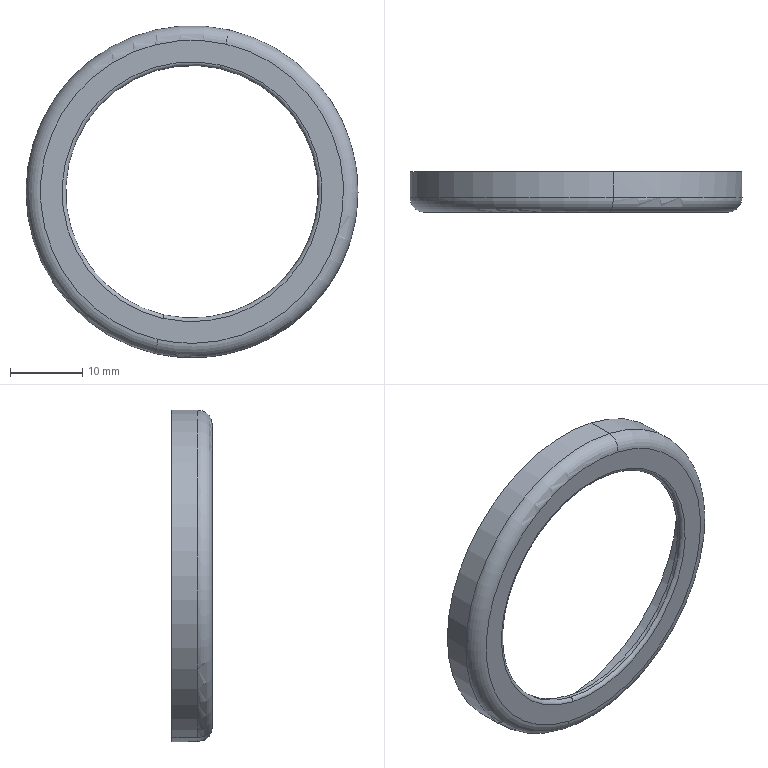Part | SolidWorks | features BaseBody 1 | 1 solid | 15 faces | box 46 x 5.6 x 46 mm | volume 1252 mm3 | torus 6 | cylinder 6 | plane 3 | commonest cylinder face diameters 35 x2 44 x2 46 x2
STEP:
#1=CARTESIAN_POINT('',(1957.701,-235.4,873.467));
#2=VERTEX_POINT('',#1);
#3=CARTESIAN_POINT('',(1948.299,-235.4,832.533));
#4=VERTEX_POINT('',#3);
#5=CARTESIAN_POINT('',(1953.,-235.4,853.));
#6=DIRECTION('',(0.,-1.,0.));
#7=DIRECTION('',(0.9746,0.,-0.2239));
#8=AXIS2_PLACEMENT_3D('',#5,#6,#7);
#9=CIRCLE('',#8,21.);
#10=EDGE_CURVE('',#2,#4,#9,.T.);
#11=ORIENTED_EDGE('',*,*,#10,.F.);
#12=CARTESIAN_POINT('',(1957.701,-235.4,873.467));
#13=CARTESIAN_POINT('',(1959.67,-235.4,873.015));
#14=CARTESIAN_POINT('',(1961.585,-235.4,872.326));
#15=CARTESIAN_POINT('',(1963.408,-235.4,871.408));
#16=CARTESIAN_POINT('',(1966.796,-235.4,869.153));
#17=CARTESIAN_POINT('',(1969.553,-235.4,866.159));
#18=CARTESIAN_POINT('',(1970.744,-235.4,864.503));
#19=CARTESIAN_POINT('',(1972.705,-235.4,860.936));
#20=CARTESIAN_POINT('',(1973.764,-235.4,857.006));
#21=CARTESIAN_POINT('',(1974.053,-235.4,854.987));
#22=CARTESIAN_POINT('',(1974.141,-235.4,850.917));
#23=CARTESIAN_POINT('',(1973.261,-235.4,846.944));
#24=CARTESIAN_POINT('',(1972.583,-235.4,845.019));
#25=CARTESIAN_POINT('',(1970.778,-235.4,841.371));
#26=CARTESIAN_POINT('',(1968.159,-235.4,838.256));
#27=CARTESIAN_POINT('',(1966.667,-235.4,836.863));
#28=CARTESIAN_POINT('',(1963.379,-235.4,834.465));
#29=CARTESIAN_POINT('',(1959.616,-235.4,832.915));
#30=CARTESIAN_POINT('',(1957.649,-235.4,832.371));
#31=CARTESIAN_POINT('',(1954.569,-235.4,831.908));
#32=CARTESIAN_POINT('',(1951.473,-235.4,832.014));
#33=CARTESIAN_POINT('',(1950.403,-235.4,832.12));
#34=CARTESIAN_POINT('',(1949.343,-235.4,832.293));
#35=CARTESIAN_POINT('',(1948.299,-235.4,832.533));
#36=B_SPLINE_CURVE_WITH_KNOTS('',5,(#12,#13,#14,#15,#16,#17,#18,#19,#20,#21,#22,#23,#24,#25,#26,#27,#28,#29,#30,#31,#32,#33,#34,#35),.UNSPECIFIED.,.F.,.F.,(6,3,3,3,3,3,3,6),(0.,0.1531,0.3063,0.4594,0.6125,0.7656,0.9188,1.),.UNSPECIFIED.);
#37=EDGE_CURVE('',#2,#4,#36,.T.);
#38=ORIENTED_EDGE('',*,*,#37,.T.);
#39=EDGE_LOOP('',(#11,#38));
#40=FACE_OUTER_BOUND('',#39,.T.);
#41=CARTESIAN_POINT('',(1956.918,-235.4,870.056));
#42=VERTEX_POINT('',#41);
#43=CARTESIAN_POINT('',(1949.082,-235.4,835.944));
#44=VERTEX_POINT('',#43);
#45=CARTESIAN_POINT('',(1956.918,-235.4,870.056));
#46=CARTESIAN_POINT('',(1958.516,-235.4,869.689));
#47=CARTESIAN_POINT('',(1960.07,-235.4,869.135));
#48=CARTESIAN_POINT('',(1961.553,-235.4,868.4));
#49=CARTESIAN_POINT('',(1964.319,-235.4,866.597));
#50=CARTESIAN_POINT('',(1966.593,-235.4,864.204));
#51=CARTESIAN_POINT('',(1967.585,-235.4,862.879));
#52=CARTESIAN_POINT('',(1969.239,-235.4,860.022));
#53=CARTESIAN_POINT('',(1970.188,-235.4,856.86));
#54=CARTESIAN_POINT('',(1970.474,-235.4,855.23));
#55=CARTESIAN_POINT('',(1970.66,-235.4,851.934));
#56=CARTESIAN_POINT('',(1970.079,-235.4,848.684));
#57=CARTESIAN_POINT('',(1969.599,-235.4,847.101));
#58=CARTESIAN_POINT('',(1968.276,-235.4,844.076));
#59=CARTESIAN_POINT('',(1966.291,-235.4,841.438));
#60=CARTESIAN_POINT('',(1965.147,-235.4,840.242));
#61=CARTESIAN_POINT('',(1962.601,-235.4,838.14));
#62=CARTESIAN_POINT('',(1959.639,-235.4,836.683));
#63=CARTESIAN_POINT('',(1958.079,-235.4,836.132));
#64=CARTESIAN_POINT('',(1955.331,-235.4,835.512));
#65=CARTESIAN_POINT('',(1952.524,-235.4,835.449));
#66=CARTESIAN_POINT('',(1951.362,-235.4,835.519));
#67=CARTESIAN_POINT('',(1950.211,-235.4,835.685));
#68=CARTESIAN_POINT('',(1949.082,-235.4,835.944));
#69=B_SPLINE_CURVE_WITH_KNOTS('',5,(#45,#46,#47,#48,#49,#50,#51,#52,#53,#54,#55,#56,#57,#58,#59,#60,#61,#62,#63,#64,#65,#66,#67,#68),.UNSPECIFIED.,.F.,.F.,(6,3,3,3,3,3,3,6),(0.,0.1491,0.2982,0.4473,0.5964,0.7455,0.8946,1.),.UNSPECIFIED.);
#70=EDGE_CURVE('',#42,#44,#69,.T.);
#71=ORIENTED_EDGE('',*,*,#70,.F.);
#72=CARTESIAN_POINT('',(1953.,-235.4,853.));
#73=DIRECTION('',(0.,-1.,0.));
#74=DIRECTION('',(0.9746,0.,-0.2239));
#75=AXIS2_PLACEMENT_3D('',#72,#73,#74);
#76=CIRCLE('',#75,17.5);
#77=EDGE_CURVE('',#42,#44,#76,.T.);
#78=ORIENTED_EDGE('',*,*,#77,.T.);
#79=EDGE_LOOP('',(#71,#78));
#80=FACE_BOUND('',#79,.T.);
#81=CARTESIAN_POINT('',(1953.,-235.4,853.));
#82=DIRECTION('',(0.,-1.,0.));
#83=DIRECTION('',(0.2239,0.,0.9746));
#84=AXIS2_PLACEMENT_3D('',#81,#82,#83);
#85=PLANE('',#84);
#86=ADVANCED_FACE('',(#40,#80),#85,.F.);
#87=ORIENTED_EDGE('',*,*,#10,.T.);
#88=CARTESIAN_POINT('',(1948.075,-234.4,831.558));
#89=VERTEX_POINT('',#88);
#90=CARTESIAN_POINT('',(1948.299,-234.4,832.533));
#91=DIRECTION('',(0.9746,0.,-0.2239));
#92=DIRECTION('',(0.,-1.,0.));
#93=AXIS2_PLACEMENT_3D('',#90,#91,#92);
#94=CIRCLE('',#93,1.);
#95=EDGE_CURVE('',#4,#89,#94,.T.);
#96=ORIENTED_EDGE('',*,*,#95,.T.);
#97=CARTESIAN_POINT('',(1957.925,-234.4,874.442));
#98=VERTEX_POINT('',#97);
#99=CARTESIAN_POINT('',(1953.,-234.4,853.));
#100=DIRECTION('',(0.,-1.,0.));
#101=DIRECTION('',(0.9746,0.,-0.2239));
#102=AXIS2_PLACEMENT_3D('',#99,#100,#101);
#103=CIRCLE('',#102,22.);
#104=EDGE_CURVE('',#98,#89,#103,.T.);
#105=ORIENTED_EDGE('',*,*,#104,.F.);
#106=CARTESIAN_POINT('',(1957.701,-234.4,873.467));
#107=DIRECTION('',(0.9746,0.,-0.2239));
#108=DIRECTION('',(0.,-1.,0.));
#109=AXIS2_PLACEMENT_3D('',#106,#107,#108);
#110=CIRCLE('',#109,1.);
#111=EDGE_CURVE('',#98,#2,#110,.T.);
#112=ORIENTED_EDGE('',*,*,#111,.T.);
#113=EDGE_LOOP('',(#87,#96,#105,#112));
#114=FACE_OUTER_BOUND('',#113,.T.);
#115=CARTESIAN_POINT('',(1953.,-234.4,853.));
#116=DIRECTION('',(0.,-1.,0.));
#117=DIRECTION('',(-0.2239,0.,-0.9746));
#118=AXIS2_PLACEMENT_3D('',#115,#116,#117);
#119=TOROIDAL_SURFACE('',#118,21.,1.);
#120=ADVANCED_FACE('',(#114),#119,.F.);
#121=CARTESIAN_POINT('',(1953.,-234.4,853.));
#122=DIRECTION('',(0.,1.,0.));
#123=DIRECTION('',(0.9746,0.,-0.2239));
#124=AXIS2_PLACEMENT_3D('',#121,#122,#123);
#125=CIRCLE('',#124,22.);
#126=EDGE_CURVE('',#98,#89,#125,.T.);
#127=ORIENTED_EDGE('',*,*,#126,.T.);
#128=ORIENTED_EDGE('',*,*,#95,.F.);
#129=ORIENTED_EDGE('',*,*,#37,.F.);
#130=ORIENTED_EDGE('',*,*,#111,.F.);
#131=EDGE_LOOP('',(#127,#128,#129,#130));
#132=FACE_OUTER_BOUND('',#131,.T.);
#133=CARTESIAN_POINT('',(1953.,-234.4,853.));
#134=DIRECTION('',(0.,-1.,0.));
#135=DIRECTION('',(0.2239,0.,0.9746));
#136=AXIS2_PLACEMENT_3D('',#133,#134,#135);
#137=TOROIDAL_SURFACE('',#136,21.,1.);
#138=ADVANCED_FACE('',(#132),#137,.F.);
#139=ORIENTED_EDGE('',*,*,#70,.T.);
#140=CARTESIAN_POINT('',(1949.082,-235.9,835.944));
#141=VERTEX_POINT('',#140);
#142=CARTESIAN_POINT('',(1949.082,-230.52,835.944));
#143=DIRECTION('',(0.,1.,0.));
#144=VECTOR('',#143,1000.);
#145=LINE('',#142,#144);
#146=EDGE_CURVE('',#141,#44,#145,.T.);
#147=ORIENTED_EDGE('',*,*,#146,.F.);
#148=CARTESIAN_POINT('',(1956.918,-235.9,870.056));
#149=VERTEX_POINT('',#148);
#150=CARTESIAN_POINT('',(1953.,-235.9,853.));
#151=DIRECTION('',(0.,1.,0.));
#152=DIRECTION('',(0.9746,0.,-0.2239));
#153=AXIS2_PLACEMENT_3D('',#150,#151,#152);
#154=CIRCLE('',#153,17.5);
#155=EDGE_CURVE('',#149,#141,#154,.T.);
#156=ORIENTED_EDGE('',*,*,#155,.F.);
#157=CARTESIAN_POINT('',(1956.918,-230.52,870.056));
#158=DIRECTION('',(0.,-1.,0.));
#159=VECTOR('',#158,1000.);
#160=LINE('',#157,#159);
#161=EDGE_CURVE('',#42,#149,#160,.T.);
#162=ORIENTED_EDGE('',*,*,#161,.F.);
#163=EDGE_LOOP('',(#139,#147,#156,#162));
#164=FACE_OUTER_BOUND('',#163,.T.);
#165=CARTESIAN_POINT('',(1953.,-230.52,853.));
#166=DIRECTION('',(0.,-1.,0.));
#167=DIRECTION('',(0.2239,0.,0.9746));
#168=AXIS2_PLACEMENT_3D('',#165,#166,#167);
#169=CYLINDRICAL_SURFACE('',#168,17.5);
#170=ADVANCED_FACE('',(#164),#169,.F.);
#171=CARTESIAN_POINT('',(1953.,-235.9,853.));
#172=DIRECTION('',(0.,-1.,0.));
#173=DIRECTION('',(0.9746,0.,-0.2239));
#174=AXIS2_PLACEMENT_3D('',#171,#172,#173);
#175=CIRCLE('',#174,17.5);
#176=EDGE_CURVE('',#149,#141,#175,.T.);
#177=ORIENTED_EDGE('',*,*,#176,.T.);
#178=ORIENTED_EDGE('',*,*,#146,.T.);
#179=ORIENTED_EDGE('',*,*,#77,.F.);
#180=ORIENTED_EDGE('',*,*,#161,.T.);
#181=EDGE_LOOP('',(#177,#178,#179,#180));
#182=FACE_OUTER_BOUND('',#181,.T.);
#183=CARTESIAN_POINT('',(1953.,-230.52,853.));
#184=DIRECTION('',(0.,-1.,0.));
#185=DIRECTION('',(-0.2239,0.,-0.9746));
#186=AXIS2_PLACEMENT_3D('',#183,#184,#185);
#187=CYLINDRICAL_SURFACE('',#186,17.5);
#188=ADVANCED_FACE('',(#182),#187,.F.);
#189=ORIENTED_EDGE('',*,*,#104,.T.);
#190=CARTESIAN_POINT('',(1948.075,-230.8,831.558));
#191=VERTEX_POINT('',#190);
#192=CARTESIAN_POINT('',(1948.075,-230.52,831.558));
#193=DIRECTION('',(0.,1.,0.));
#194=VECTOR('',#193,1000.);
#195=LINE('',#192,#194);
#196=EDGE_CURVE('',#89,#191,#195,.T.);
#197=ORIENTED_EDGE('',*,*,#196,.T.);
#198=CARTESIAN_POINT('',(1957.925,-230.8,874.442));
#199=VERTEX_POINT('',#198);
#200=CARTESIAN_POINT('',(1953.,-230.8,853.));
#201=DIRECTION('',(0.,-1.,0.));
#202=DIRECTION('',(0.9746,0.,-0.2239));
#203=AXIS2_PLACEMENT_3D('',#200,#201,#202);
#204=CIRCLE('',#203,22.);
#205=EDGE_CURVE('',#199,#191,#204,.T.);
#206=ORIENTED_EDGE('',*,*,#205,.F.);
#207=CARTESIAN_POINT('',(1957.925,-230.52,874.442));
#208=DIRECTION('',(0.,-1.,0.));
#209=VECTOR('',#208,1000.);
#210=LINE('',#207,#209);
#211=EDGE_CURVE('',#199,#98,#210,.T.);
#212=ORIENTED_EDGE('',*,*,#211,.T.);
#213=EDGE_LOOP('',(#189,#197,#206,#212));
#214=FACE_OUTER_BOUND('',#213,.T.);
#215=CARTESIAN_POINT('',(1953.,-230.52,853.));
#216=DIRECTION('',(0.,-1.,0.));
#217=DIRECTION('',(-0.2239,0.,-0.9746));
#218=AXIS2_PLACEMENT_3D('',#215,#216,#217);
#219=CYLINDRICAL_SURFACE('',#218,22.);
#220=ADVANCED_FACE('',(#214),#219,.F.);
#221=CARTESIAN_POINT('',(1953.,-230.8,853.));
#222=DIRECTION('',(0.,1.,0.));
#223=DIRECTION('',(0.9746,0.,-0.2239));
#224=AXIS2_PLACEMENT_3D('',#221,#222,#223);
#225=CIRCLE('',#224,22.);
#226=EDGE_CURVE('',#199,#191,#225,.T.);
#227=ORIENTED_EDGE('',*,*,#226,.T.);
#228=ORIENTED_EDGE('',*,*,#196,.F.);
#229=ORIENTED_EDGE('',*,*,#126,.F.);
#230=ORIENTED_EDGE('',*,*,#211,.F.);
#231=EDGE_LOOP('',(#227,#228,#229,#230));
#232=FACE_OUTER_BOUND('',#231,.T.);
#233=CARTESIAN_POINT('',(1953.,-230.52,853.));
#234=DIRECTION('',(0.,-1.,0.));
#235=DIRECTION('',(0.2239,0.,0.9746));
#236=AXIS2_PLACEMENT_3D('',#233,#234,#235);
#237=CYLINDRICAL_SURFACE('',#236,22.);
#238=ADVANCED_FACE('',(#232),#237,.F.);
#239=ORIENTED_EDGE('',*,*,#155,.T.);
#240=CARTESIAN_POINT('',(1948.97,-236.4,835.457));
#241=VERTEX_POINT('',#240);
#242=CARTESIAN_POINT('',(1948.97,-235.9,835.457));
#243=DIRECTION('',(-0.9746,0.,0.2239));
#244=DIRECTION('',(0.,-1.,0.));
#245=AXIS2_PLACEMENT_3D('',#242,#243,#244);
#246=CIRCLE('',#245,0.5);
#247=EDGE_CURVE('',#241,#141,#246,.T.);
#248=ORIENTED_EDGE('',*,*,#247,.F.);
#249=CARTESIAN_POINT('',(1957.03,-236.4,870.543));
#250=VERTEX_POINT('',#249);
#251=CARTESIAN_POINT('',(1953.,-236.4,853.));
#252=DIRECTION('',(0.,1.,0.));
#253=DIRECTION('',(0.9746,0.,-0.2239));
#254=AXIS2_PLACEMENT_3D('',#251,#252,#253);
#255=CIRCLE('',#254,18.);
#256=EDGE_CURVE('',#250,#241,#255,.T.);
#257=ORIENTED_EDGE('',*,*,#256,.F.);
#258=CARTESIAN_POINT('',(1957.03,-235.9,870.543));
#259=DIRECTION('',(-0.9746,0.,0.2239));
#260=DIRECTION('',(0.,-1.,0.));
#261=AXIS2_PLACEMENT_3D('',#258,#259,#260);
#262=CIRCLE('',#261,0.5);
#263=EDGE_CURVE('',#149,#250,#262,.T.);
#264=ORIENTED_EDGE('',*,*,#263,.F.);
#265=EDGE_LOOP('',(#239,#248,#257,#264));
#266=FACE_OUTER_BOUND('',#265,.T.);
#267=CARTESIAN_POINT('',(1953.,-235.9,853.));
#268=DIRECTION('',(0.,-1.,0.));
#269=DIRECTION('',(0.2239,0.,0.9746));
#270=AXIS2_PLACEMENT_3D('',#267,#268,#269);
#271=TOROIDAL_SURFACE('',#270,18.,0.5);
#272=ADVANCED_FACE('',(#266),#271,.T.);
#273=CARTESIAN_POINT('',(1953.,-236.4,853.));
#274=DIRECTION('',(0.,-1.,0.));
#275=DIRECTION('',(0.9746,0.,-0.2239));
#276=AXIS2_PLACEMENT_3D('',#273,#274,#275);
#277=CIRCLE('',#276,18.);
#278=EDGE_CURVE('',#250,#241,#277,.T.);
#279=ORIENTED_EDGE('',*,*,#278,.T.);
#280=ORIENTED_EDGE('',*,*,#247,.T.);
#281=ORIENTED_EDGE('',*,*,#176,.F.);
#282=ORIENTED_EDGE('',*,*,#263,.T.);
#283=EDGE_LOOP('',(#279,#280,#281,#282));
#284=FACE_OUTER_BOUND('',#283,.T.);
#285=CARTESIAN_POINT('',(1953.,-235.9,853.));
#286=DIRECTION('',(0.,-1.,0.));
#287=DIRECTION('',(-0.2239,0.,-0.9746));
#288=AXIS2_PLACEMENT_3D('',#285,#286,#287);
#289=TOROIDAL_SURFACE('',#288,18.,0.5);
#290=ADVANCED_FACE('',(#284),#289,.T.);
#291=CARTESIAN_POINT('',(1958.149,-230.8,875.416));
#292=VERTEX_POINT('',#291);
#293=CARTESIAN_POINT('',(1947.851,-230.8,830.584));
#294=VERTEX_POINT('',#293);
#295=CARTESIAN_POINT('',(1953.,-230.8,853.));
#296=DIRECTION('',(0.,-1.,0.));
#297=DIRECTION('',(0.9746,0.,-0.2239));
#298=AXIS2_PLACEMENT_3D('',#295,#296,#297);
#299=CIRCLE('',#298,23.);
#300=EDGE_CURVE('',#292,#294,#299,.T.);
#301=ORIENTED_EDGE('',*,*,#300,.F.);
#302=CARTESIAN_POINT('',(1958.149,-230.8,875.416));
#303=CARTESIAN_POINT('',(1960.21,-230.8,874.943));
#304=CARTESIAN_POINT('',(1962.216,-230.8,874.233));
#305=CARTESIAN_POINT('',(1964.132,-230.8,873.294));
#306=CARTESIAN_POINT('',(1967.713,-230.8,870.993));
#307=CARTESIAN_POINT('',(1970.68,-230.8,867.94));
#308=CARTESIAN_POINT('',(1971.98,-230.8,866.248));
#309=CARTESIAN_POINT('',(1974.169,-230.8,862.598));
#310=CARTESIAN_POINT('',(1975.473,-230.8,858.545));
#311=CARTESIAN_POINT('',(1975.888,-230.8,856.453));
#312=CARTESIAN_POINT('',(1976.23,-230.8,852.209));
#313=CARTESIAN_POINT('',(1975.6,-230.8,847.999));
#314=CARTESIAN_POINT('',(1975.044,-230.8,845.94));
#315=CARTESIAN_POINT('',(1973.467,-230.8,841.985));
#316=CARTESIAN_POINT('',(1971.035,-230.8,838.492));
#317=CARTESIAN_POINT('',(1969.623,-230.8,836.893));
#318=CARTESIAN_POINT('',(1966.456,-230.8,834.048));
#319=CARTESIAN_POINT('',(1962.727,-230.8,831.996));
#320=CARTESIAN_POINT('',(1960.751,-230.8,831.19));
#321=CARTESIAN_POINT('',(1956.991,-230.8,830.14));
#322=CARTESIAN_POINT('',(1953.102,-230.8,829.898));
#323=CARTESIAN_POINT('',(1951.328,-230.8,829.959));
#324=CARTESIAN_POINT('',(1949.57,-230.8,830.189));
#325=CARTESIAN_POINT('',(1947.851,-230.8,830.584));
#326=B_SPLINE_CURVE_WITH_KNOTS('',5,(#302,#303,#304,#305,#306,#307,#308,#309,#310,#311,#312,#313,#314,#315,#316,#317,#318,#319,#320,#321,#322,#323,#324,#325),.UNSPECIFIED.,.F.,.F.,(6,3,3,3,3,3,3,6),(0.,0.1463,0.2926,0.439,0.5853,0.7316,0.8779,1.),.UNSPECIFIED.);
#327=EDGE_CURVE('',#292,#294,#326,.T.);
#328=ORIENTED_EDGE('',*,*,#327,.T.);
#329=EDGE_LOOP('',(#301,#328));
#330=FACE_OUTER_BOUND('',#329,.T.);
#331=ORIENTED_EDGE('',*,*,#226,.F.);
#332=ORIENTED_EDGE('',*,*,#205,.T.);
#333=EDGE_LOOP('',(#331,#332));
#334=FACE_BOUND('',#333,.T.);
#335=CARTESIAN_POINT('',(1953.,-230.8,853.));
#336=DIRECTION('',(0.,-1.,0.));
#337=DIRECTION('',(0.2239,0.,0.9746));
#338=AXIS2_PLACEMENT_3D('',#335,#336,#337);
#339=PLANE('',#338);
#340=ADVANCED_FACE('',(#330,#334),#339,.F.);
#341=CARTESIAN_POINT('',(1957.701,-236.4,873.467));
#342=VERTEX_POINT('',#341);
#343=CARTESIAN_POINT('',(1948.299,-236.4,832.533));
#344=VERTEX_POINT('',#343);
#345=CARTESIAN_POINT('',(1957.701,-236.4,873.467));
#346=CARTESIAN_POINT('',(1959.67,-236.4,873.015));
#347=CARTESIAN_POINT('',(1961.585,-236.4,872.326));
#348=CARTESIAN_POINT('',(1963.408,-236.4,871.408));
#349=CARTESIAN_POINT('',(1966.796,-236.4,869.153));
#350=CARTESIAN_POINT('',(1969.553,-236.4,866.159));
#351=CARTESIAN_POINT('',(1970.744,-236.4,864.503));
#352=CARTESIAN_POINT('',(1972.705,-236.4,860.936));
#353=CARTESIAN_POINT('',(1973.764,-236.4,857.006));
#354=CARTESIAN_POINT('',(1974.053,-236.4,854.987));
#355=CARTESIAN_POINT('',(1974.141,-236.4,850.917));
#356=CARTESIAN_POINT('',(1973.261,-236.4,846.944));
#357=CARTESIAN_POINT('',(1972.583,-236.4,845.019));
#358=CARTESIAN_POINT('',(1970.778,-236.4,841.371));
#359=CARTESIAN_POINT('',(1968.159,-236.4,838.256));
#360=CARTESIAN_POINT('',(1966.667,-236.4,836.863));
#361=CARTESIAN_POINT('',(1963.379,-236.4,834.465));
#362=CARTESIAN_POINT('',(1959.616,-236.4,832.915));
#363=CARTESIAN_POINT('',(1957.649,-236.4,832.371));
#364=CARTESIAN_POINT('',(1954.569,-236.4,831.908));
#365=CARTESIAN_POINT('',(1951.473,-236.4,832.014));
#366=CARTESIAN_POINT('',(1950.403,-236.4,832.12));
#367=CARTESIAN_POINT('',(1949.343,-236.4,832.293));
#368=CARTESIAN_POINT('',(1948.299,-236.4,832.533));
#369=B_SPLINE_CURVE_WITH_KNOTS('',5,(#345,#346,#347,#348,#349,#350,#351,#352,#353,#354,#355,#356,#357,#358,#359,#360,#361,#362,#363,#364,#365,#366,#367,#368),.UNSPECIFIED.,.F.,.F.,(6,3,3,3,3,3,3,6),(0.,0.1531,0.3063,0.4594,0.6125,0.7656,0.9188,1.),.UNSPECIFIED.);
#370=EDGE_CURVE('',#342,#344,#369,.T.);
#371=ORIENTED_EDGE('',*,*,#370,.F.);
#372=CARTESIAN_POINT('',(1953.,-236.4,853.));
#373=DIRECTION('',(0.,-1.,0.));
#374=DIRECTION('',(0.9746,0.,-0.2239));
#375=AXIS2_PLACEMENT_3D('',#372,#373,#374);
#376=CIRCLE('',#375,21.);
#377=EDGE_CURVE('',#342,#344,#376,.T.);
#378=ORIENTED_EDGE('',*,*,#377,.T.);
#379=EDGE_LOOP('',(#371,#378));
#380=FACE_OUTER_BOUND('',#379,.T.);
#381=ORIENTED_EDGE('',*,*,#278,.F.);
#382=ORIENTED_EDGE('',*,*,#256,.T.);
#383=EDGE_LOOP('',(#381,#382));
#384=FACE_BOUND('',#383,.T.);
#385=CARTESIAN_POINT('',(1953.,-236.4,853.));
#386=DIRECTION('',(0.,-1.,0.));
#387=DIRECTION('',(0.2239,0.,0.9746));
#388=AXIS2_PLACEMENT_3D('',#385,#386,#387);
#389=PLANE('',#388);
#390=ADVANCED_FACE('',(#380,#384),#389,.T.);
#391=ORIENTED_EDGE('',*,*,#300,.T.);
#392=CARTESIAN_POINT('',(1947.851,-234.4,830.584));
#393=VERTEX_POINT('',#392);
#394=CARTESIAN_POINT('',(1947.851,-230.52,830.584));
#395=DIRECTION('',(0.,-1.,0.));
#396=VECTOR('',#395,1000.);
#397=LINE('',#394,#396);
#398=EDGE_CURVE('',#294,#393,#397,.T.);
#399=ORIENTED_EDGE('',*,*,#398,.T.);
#400=CARTESIAN_POINT('',(1958.149,-234.4,875.416));
#401=VERTEX_POINT('',#400);
#402=CARTESIAN_POINT('',(1953.,-234.4,853.));
#403=DIRECTION('',(0.,-1.,0.));
#404=DIRECTION('',(0.9746,0.,-0.2239));
#405=AXIS2_PLACEMENT_3D('',#402,#403,#404);
#406=CIRCLE('',#405,23.);
#407=EDGE_CURVE('',#401,#393,#406,.T.);
#408=ORIENTED_EDGE('',*,*,#407,.F.);
#409=CARTESIAN_POINT('',(1958.149,-230.52,875.416));
#410=DIRECTION('',(0.,1.,0.));
#411=VECTOR('',#410,1000.);
#412=LINE('',#409,#411);
#413=EDGE_CURVE('',#401,#292,#412,.T.);
#414=ORIENTED_EDGE('',*,*,#413,.T.);
#415=EDGE_LOOP('',(#391,#399,#408,#414));
#416=FACE_OUTER_BOUND('',#415,.T.);
#417=CARTESIAN_POINT('',(1953.,-230.52,853.));
#418=DIRECTION('',(0.,-1.,0.));
#419=DIRECTION('',(-0.2239,0.,-0.9746));
#420=AXIS2_PLACEMENT_3D('',#417,#418,#419);
#421=CYLINDRICAL_SURFACE('',#420,23.);
#422=ADVANCED_FACE('',(#416),#421,.T.);
#423=CARTESIAN_POINT('',(1953.,-234.4,853.));
#424=DIRECTION('',(0.,1.,0.));
#425=DIRECTION('',(0.9746,0.,-0.2239));
#426=AXIS2_PLACEMENT_3D('',#423,#424,#425);
#427=CIRCLE('',#426,23.);
#428=EDGE_CURVE('',#401,#393,#427,.T.);
#429=ORIENTED_EDGE('',*,*,#428,.T.);
#430=ORIENTED_EDGE('',*,*,#398,.F.);
#431=ORIENTED_EDGE('',*,*,#327,.F.);
#432=ORIENTED_EDGE('',*,*,#413,.F.);
#433=EDGE_LOOP('',(#429,#430,#431,#432));
#434=FACE_OUTER_BOUND('',#433,.T.);
#435=CARTESIAN_POINT('',(1953.,-230.52,853.));
#436=DIRECTION('',(0.,-1.,0.));
#437=DIRECTION('',(0.2239,0.,0.9746));
#438=AXIS2_PLACEMENT_3D('',#435,#436,#437);
#439=CYLINDRICAL_SURFACE('',#438,23.);
#440=ADVANCED_FACE('',(#434),#439,.T.);
#441=ORIENTED_EDGE('',*,*,#370,.T.);
#442=CARTESIAN_POINT('',(1948.299,-234.4,832.533));
#443=DIRECTION('',(-0.9746,0.,0.2239));
#444=DIRECTION('',(0.,-1.,0.));
#445=AXIS2_PLACEMENT_3D('',#442,#443,#444);
#446=CIRCLE('',#445,2.);
#447=EDGE_CURVE('',#393,#344,#446,.T.);
#448=ORIENTED_EDGE('',*,*,#447,.F.);
#449=ORIENTED_EDGE('',*,*,#428,.F.);
#450=CARTESIAN_POINT('',(1957.701,-234.4,873.467));
#451=DIRECTION('',(-0.9746,0.,0.2239));
#452=DIRECTION('',(0.,-1.,0.));
#453=AXIS2_PLACEMENT_3D('',#450,#451,#452);
#454=CIRCLE('',#453,2.);
#455=EDGE_CURVE('',#342,#401,#454,.T.);
#456=ORIENTED_EDGE('',*,*,#455,.F.);
#457=EDGE_LOOP('',(#441,#448,#449,#456));
#458=FACE_OUTER_BOUND('',#457,.T.);
#459=CARTESIAN_POINT('',(1953.,-234.4,853.));
#460=DIRECTION('',(0.,-1.,0.));
#461=DIRECTION('',(0.2239,0.,0.9746));
#462=AXIS2_PLACEMENT_3D('',#459,#460,#461);
#463=TOROIDAL_SURFACE('',#462,21.,2.);
#464=ADVANCED_FACE('',(#458),#463,.T.);
#465=ORIENTED_EDGE('',*,*,#407,.T.);
#466=ORIENTED_EDGE('',*,*,#447,.T.);
#467=ORIENTED_EDGE('',*,*,#377,.F.);
#468=ORIENTED_EDGE('',*,*,#455,.T.);
#469=EDGE_LOOP('',(#465,#466,#467,#468));
#470=FACE_OUTER_BOUND('',#469,.T.);
#471=CARTESIAN_POINT('',(1953.,-234.4,853.));
#472=DIRECTION('',(0.,-1.,0.));
#473=DIRECTION('',(-0.2239,0.,-0.9746));
#474=AXIS2_PLACEMENT_3D('',#471,#472,#473);
#475=TOROIDAL_SURFACE('',#474,21.,2.);
#476=ADVANCED_FACE('',(#470),#475,.T.);
#477=CLOSED_SHELL('',(#86,#120,#138,#170,#188,#220,#238,#272,#290,#340,#390,#422,#440,#464,#476));
#478=MANIFOLD_SOLID_BREP('',#477);
#479=CARTESIAN_POINT('',(0.,0.,0.));
#480=DIRECTION('',(0.,0.,1.));
#481=DIRECTION('',(1.,0.,0.));
#482=AXIS2_PLACEMENT_3D('',#479,#480,#481);
#483=(LENGTH_UNIT()NAMED_UNIT(*)SI_UNIT(.MILLI.,.METRE.));
#484=UNCERTAINTY_MEASURE_WITH_UNIT(LENGTH_MEASURE(0.00001),#483,'','');
#485=(NAMED_UNIT(*)PLANE_ANGLE_UNIT()SI_UNIT($,.RADIAN.));
#486=(NAMED_UNIT(*)SI_UNIT($,.STERADIAN.)SOLID_ANGLE_UNIT());
#487=(GEOMETRIC_REPRESENTATION_CONTEXT(3)GLOBAL_UNCERTAINTY_ASSIGNED_CONTEXT((#484))GLOBAL_UNIT_ASSIGNED_CONTEXT((#483,#485,#486))REPRESENTATION_CONTEXT('',''));
#488=ADVANCED_BREP_SHAPE_REPRESENTATION('',(#478,#482),#487);